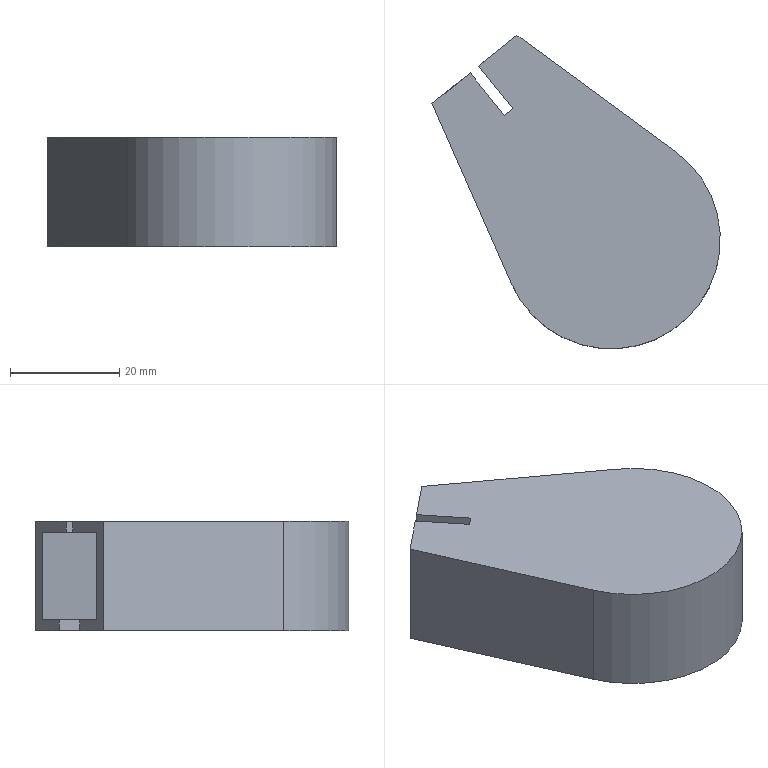Part | SolidWorks | features Cut 2, Extrusion 1, Shell 1 | 1 solid | 18 faces | box 52.852 x 57.443 x 20 mm | volume 11809 mm3 | plane 16 | cylinder 2 | commonest cylinder face diameters 36 x1 40 x1
STEP:
#1=CARTESIAN_POINT('',(-25.837,30.553,18.));
#2=VERTEX_POINT('',#1);
#3=CARTESIAN_POINT('',(-25.837,30.553,20.));
#4=VERTEX_POINT('',#3);
#5=CARTESIAN_POINT('',(-25.837,30.553,20.));
#6=DIRECTION('',(0.,0.,1.));
#7=VECTOR('',#6,1000.);
#8=LINE('',#5,#7);
#9=EDGE_CURVE('',#2,#4,#8,.T.);
#10=ORIENTED_EDGE('',*,*,#9,.F.);
#11=CARTESIAN_POINT('',(-31.238,26.212,18.));
#12=VERTEX_POINT('',#11);
#13=CARTESIAN_POINT('',(-25.057,31.179,18.));
#14=DIRECTION('',(0.7795,0.6264,0.));
#15=VECTOR('',#14,1000.);
#16=LINE('',#13,#15);
#17=EDGE_CURVE('',#12,#2,#16,.T.);
#18=ORIENTED_EDGE('',*,*,#17,.F.);
#19=CARTESIAN_POINT('',(-31.238,26.212,2.));
#20=VERTEX_POINT('',#19);
#21=CARTESIAN_POINT('',(-31.238,26.212,20.));
#22=DIRECTION('',(0.,0.,-1.));
#23=VECTOR('',#22,1000.);
#24=LINE('',#21,#23);
#25=EDGE_CURVE('',#12,#20,#24,.T.);
#26=ORIENTED_EDGE('',*,*,#25,.T.);
#27=CARTESIAN_POINT('',(-27.396,29.3,2.));
#28=VERTEX_POINT('',#27);
#29=CARTESIAN_POINT('',(-25.057,31.179,2.));
#30=DIRECTION('',(0.7795,0.6264,0.));
#31=VECTOR('',#30,1000.);
#32=LINE('',#29,#31);
#33=EDGE_CURVE('',#20,#28,#32,.T.);
#34=ORIENTED_EDGE('',*,*,#33,.T.);
#35=CARTESIAN_POINT('',(-27.396,29.3,0.));
#36=VERTEX_POINT('',#35);
#37=CARTESIAN_POINT('',(-27.396,29.3,20.001));
#38=DIRECTION('',(0.,0.,-1.));
#39=VECTOR('',#38,1000.);
#40=LINE('',#37,#39);
#41=EDGE_CURVE('',#28,#36,#40,.T.);
#42=ORIENTED_EDGE('',*,*,#41,.T.);
#43=CARTESIAN_POINT('',(-32.852,24.915,0.));
#44=VERTEX_POINT('',#43);
#45=CARTESIAN_POINT('',(-25.057,31.179,0.));
#46=DIRECTION('',(0.7795,0.6264,0.));
#47=VECTOR('',#46,1000.);
#48=LINE('',#45,#47);
#49=EDGE_CURVE('',#44,#36,#48,.T.);
#50=ORIENTED_EDGE('',*,*,#49,.F.);
#51=CARTESIAN_POINT('',(-32.852,24.915,20.));
#52=VERTEX_POINT('',#51);
#53=CARTESIAN_POINT('',(-32.852,24.915,20.));
#54=DIRECTION('',(0.,0.,-1.));
#55=VECTOR('',#54,1000.);
#56=LINE('',#53,#55);
#57=EDGE_CURVE('',#52,#44,#56,.T.);
#58=ORIENTED_EDGE('',*,*,#57,.F.);
#59=CARTESIAN_POINT('',(-25.057,31.179,20.));
#60=DIRECTION('',(0.7795,0.6264,0.));
#61=VECTOR('',#60,1000.);
#62=LINE('',#59,#61);
#63=EDGE_CURVE('',#52,#4,#62,.T.);
#64=ORIENTED_EDGE('',*,*,#63,.T.);
#65=EDGE_LOOP('',(#10,#18,#26,#34,#42,#50,#58,#64));
#66=FACE_OUTER_BOUND('',#65,.T.);
#67=CARTESIAN_POINT('',(-25.057,31.179,20.));
#68=DIRECTION('',(-0.6264,0.7795,0.));
#69=DIRECTION('',(-0.7795,-0.6264,0.));
#70=AXIS2_PLACEMENT_3D('',#67,#68,#69);
#71=PLANE('',#70);
#72=ADVANCED_FACE('',(#66),#71,.T.);
#73=CARTESIAN_POINT('',(-24.278,31.806,20.));
#74=VERTEX_POINT('',#73);
#75=CARTESIAN_POINT('',(-24.278,31.806,18.));
#76=VERTEX_POINT('',#75);
#77=CARTESIAN_POINT('',(-24.278,31.806,20.));
#78=DIRECTION('',(0.,0.,-1.));
#79=VECTOR('',#78,1000.);
#80=LINE('',#77,#79);
#81=EDGE_CURVE('',#74,#76,#80,.T.);
#82=ORIENTED_EDGE('',*,*,#81,.F.);
#83=CARTESIAN_POINT('',(-17.262,37.443,20.));
#84=VERTEX_POINT('',#83);
#85=CARTESIAN_POINT('',(-25.057,31.179,20.));
#86=DIRECTION('',(0.7795,0.6264,0.));
#87=VECTOR('',#86,1000.);
#88=LINE('',#85,#87);
#89=EDGE_CURVE('',#74,#84,#88,.T.);
#90=ORIENTED_EDGE('',*,*,#89,.T.);
#91=CARTESIAN_POINT('',(-17.262,37.443,0.));
#92=VERTEX_POINT('',#91);
#93=CARTESIAN_POINT('',(-17.262,37.443,20.));
#94=DIRECTION('',(0.,0.,-1.));
#95=VECTOR('',#94,1000.);
#96=LINE('',#93,#95);
#97=EDGE_CURVE('',#84,#92,#96,.T.);
#98=ORIENTED_EDGE('',*,*,#97,.T.);
#99=CARTESIAN_POINT('',(-22.719,33.058,0.));
#100=VERTEX_POINT('',#99);
#101=CARTESIAN_POINT('',(-25.057,31.179,0.));
#102=DIRECTION('',(0.7795,0.6264,0.));
#103=VECTOR('',#102,1000.);
#104=LINE('',#101,#103);
#105=EDGE_CURVE('',#100,#92,#104,.T.);
#106=ORIENTED_EDGE('',*,*,#105,.F.);
#107=CARTESIAN_POINT('',(-22.719,33.058,2.));
#108=VERTEX_POINT('',#107);
#109=CARTESIAN_POINT('',(-22.719,33.058,20.001));
#110=DIRECTION('',(0.,0.,1.));
#111=VECTOR('',#110,1000.);
#112=LINE('',#109,#111);
#113=EDGE_CURVE('',#100,#108,#112,.T.);
#114=ORIENTED_EDGE('',*,*,#113,.T.);
#115=CARTESIAN_POINT('',(-18.876,36.146,2.));
#116=VERTEX_POINT('',#115);
#117=CARTESIAN_POINT('',(-25.057,31.179,2.));
#118=DIRECTION('',(0.7795,0.6264,0.));
#119=VECTOR('',#118,1000.);
#120=LINE('',#117,#119);
#121=EDGE_CURVE('',#108,#116,#120,.T.);
#122=ORIENTED_EDGE('',*,*,#121,.T.);
#123=CARTESIAN_POINT('',(-18.876,36.146,18.));
#124=VERTEX_POINT('',#123);
#125=CARTESIAN_POINT('',(-18.876,36.146,20.));
#126=DIRECTION('',(0.,0.,-1.));
#127=VECTOR('',#126,1000.);
#128=LINE('',#125,#127);
#129=EDGE_CURVE('',#124,#116,#128,.T.);
#130=ORIENTED_EDGE('',*,*,#129,.F.);
#131=CARTESIAN_POINT('',(-25.057,31.179,18.));
#132=DIRECTION('',(0.7795,0.6264,0.));
#133=VECTOR('',#132,1000.);
#134=LINE('',#131,#133);
#135=EDGE_CURVE('',#76,#124,#134,.T.);
#136=ORIENTED_EDGE('',*,*,#135,.F.);
#137=EDGE_LOOP('',(#82,#90,#98,#106,#114,#122,#130,#136));
#138=FACE_OUTER_BOUND('',#137,.T.);
#139=CARTESIAN_POINT('',(-25.057,31.179,20.));
#140=DIRECTION('',(-0.6264,0.7795,0.));
#141=DIRECTION('',(-0.7795,-0.6264,0.));
#142=AXIS2_PLACEMENT_3D('',#139,#140,#141);
#143=PLANE('',#142);
#144=ADVANCED_FACE('',(#138),#143,.T.);
#145=CARTESIAN_POINT('',(-18.298,-8.073,0.));
#146=VERTEX_POINT('',#145);
#147=CARTESIAN_POINT('',(-18.298,-8.073,0.));
#148=DIRECTION('',(-0.4036,0.9149,0.));
#149=VECTOR('',#148,1000.);
#150=LINE('',#147,#149);
#151=EDGE_CURVE('',#146,#44,#150,.T.);
#152=ORIENTED_EDGE('',*,*,#151,.F.);
#153=CARTESIAN_POINT('',(-18.298,-8.073,20.));
#154=VERTEX_POINT('',#153);
#155=CARTESIAN_POINT('',(-18.298,-8.073,20.));
#156=DIRECTION('',(0.,0.,-1.));
#157=VECTOR('',#156,1000.);
#158=LINE('',#155,#157);
#159=EDGE_CURVE('',#154,#146,#158,.T.);
#160=ORIENTED_EDGE('',*,*,#159,.F.);
#161=CARTESIAN_POINT('',(-18.298,-8.073,20.));
#162=DIRECTION('',(-0.4036,0.9149,0.));
#163=VECTOR('',#162,1000.);
#164=LINE('',#161,#163);
#165=EDGE_CURVE('',#154,#52,#164,.T.);
#166=ORIENTED_EDGE('',*,*,#165,.T.);
#167=ORIENTED_EDGE('',*,*,#57,.T.);
#168=EDGE_LOOP('',(#152,#160,#166,#167));
#169=FACE_OUTER_BOUND('',#168,.T.);
#170=CARTESIAN_POINT('',(-18.298,-8.073,20.));
#171=DIRECTION('',(-0.9149,-0.4036,0.));
#172=DIRECTION('',(0.4036,-0.9149,0.));
#173=AXIS2_PLACEMENT_3D('',#170,#171,#172);
#174=PLANE('',#173);
#175=ADVANCED_FACE('',(#169),#174,.T.);
#176=CARTESIAN_POINT('',(11.821,16.133,0.));
#177=VERTEX_POINT('',#176);
#178=CARTESIAN_POINT('',(0.,0.,0.));
#179=DIRECTION('',(0.,0.,1.));
#180=DIRECTION('',(1.,0.,0.));
#181=AXIS2_PLACEMENT_3D('',#178,#179,#180);
#182=CIRCLE('',#181,20.);
#183=EDGE_CURVE('',#146,#177,#182,.T.);
#184=ORIENTED_EDGE('',*,*,#183,.T.);
#185=CARTESIAN_POINT('',(11.821,16.133,20.));
#186=VERTEX_POINT('',#185);
#187=CARTESIAN_POINT('',(11.821,16.133,20.));
#188=DIRECTION('',(0.,0.,-1.));
#189=VECTOR('',#188,1000.);
#190=LINE('',#187,#189);
#191=EDGE_CURVE('',#186,#177,#190,.T.);
#192=ORIENTED_EDGE('',*,*,#191,.F.);
#193=CARTESIAN_POINT('',(0.,0.,20.));
#194=DIRECTION('',(0.,0.,1.));
#195=DIRECTION('',(1.,0.,0.));
#196=AXIS2_PLACEMENT_3D('',#193,#194,#195);
#197=CIRCLE('',#196,20.);
#198=EDGE_CURVE('',#154,#186,#197,.T.);
#199=ORIENTED_EDGE('',*,*,#198,.F.);
#200=ORIENTED_EDGE('',*,*,#159,.T.);
#201=EDGE_LOOP('',(#184,#192,#199,#200));
#202=FACE_OUTER_BOUND('',#201,.T.);
#203=CARTESIAN_POINT('',(0.,0.,20.));
#204=DIRECTION('',(0.,0.,-1.));
#205=DIRECTION('',(-1.,0.,0.));
#206=AXIS2_PLACEMENT_3D('',#203,#204,#205);
#207=CYLINDRICAL_SURFACE('',#206,20.);
#208=ADVANCED_FACE('',(#202),#207,.T.);
#209=CARTESIAN_POINT('',(11.821,16.133,0.));
#210=DIRECTION('',(0.8066,-0.5911,0.));
#211=VECTOR('',#210,1000.);
#212=LINE('',#209,#211);
#213=EDGE_CURVE('',#92,#177,#212,.T.);
#214=ORIENTED_EDGE('',*,*,#213,.F.);
#215=ORIENTED_EDGE('',*,*,#97,.F.);
#216=CARTESIAN_POINT('',(11.821,16.133,20.));
#217=DIRECTION('',(0.8066,-0.5911,0.));
#218=VECTOR('',#217,1000.);
#219=LINE('',#216,#218);
#220=EDGE_CURVE('',#84,#186,#219,.T.);
#221=ORIENTED_EDGE('',*,*,#220,.T.);
#222=ORIENTED_EDGE('',*,*,#191,.T.);
#223=EDGE_LOOP('',(#214,#215,#221,#222));
#224=FACE_OUTER_BOUND('',#223,.T.);
#225=CARTESIAN_POINT('',(11.821,16.133,20.));
#226=DIRECTION('',(0.5911,0.8066,0.));
#227=DIRECTION('',(-0.8066,0.5911,0.));
#228=AXIS2_PLACEMENT_3D('',#225,#226,#227);
#229=PLANE('',#228);
#230=ADVANCED_FACE('',(#224),#229,.T.);
#231=CARTESIAN_POINT('',(-19.571,22.756,20.));
#232=VERTEX_POINT('',#231);
#233=CARTESIAN_POINT('',(-514.126,638.139,20.));
#234=DIRECTION('',(0.6264,-0.7795,0.));
#235=VECTOR('',#234,1000.);
#236=LINE('',#233,#235);
#237=EDGE_CURVE('',#4,#232,#236,.T.);
#238=ORIENTED_EDGE('',*,*,#237,.F.);
#239=ORIENTED_EDGE('',*,*,#63,.F.);
#240=ORIENTED_EDGE('',*,*,#165,.F.);
#241=ORIENTED_EDGE('',*,*,#198,.T.);
#242=ORIENTED_EDGE('',*,*,#220,.F.);
#243=ORIENTED_EDGE('',*,*,#89,.F.);
#244=CARTESIAN_POINT('',(-18.012,24.009,20.));
#245=VERTEX_POINT('',#244);
#246=CARTESIAN_POINT('',(-18.012,24.009,20.));
#247=DIRECTION('',(-0.6264,0.7795,0.));
#248=VECTOR('',#247,1000.);
#249=LINE('',#246,#248);
#250=EDGE_CURVE('',#245,#74,#249,.T.);
#251=ORIENTED_EDGE('',*,*,#250,.F.);
#252=CARTESIAN_POINT('',(-19.571,22.756,20.));
#253=DIRECTION('',(0.7795,0.6264,0.));
#254=VECTOR('',#253,1000.);
#255=LINE('',#252,#254);
#256=EDGE_CURVE('',#232,#245,#255,.T.);
#257=ORIENTED_EDGE('',*,*,#256,.F.);
#258=EDGE_LOOP('',(#238,#239,#240,#241,#242,#243,#251,#257));
#259=FACE_OUTER_BOUND('',#258,.T.);
#260=CARTESIAN_POINT('',(0.,0.,20.));
#261=DIRECTION('',(0.,0.,1.));
#262=DIRECTION('',(1.,0.,0.));
#263=AXIS2_PLACEMENT_3D('',#260,#261,#262);
#264=PLANE('',#263);
#265=ADVANCED_FACE('',(#259),#264,.T.);
#266=CARTESIAN_POINT('',(-16.454,25.264,0.));
#267=VERTEX_POINT('',#266);
#268=CARTESIAN_POINT('',(-21.131,21.505,0.));
#269=VERTEX_POINT('',#268);
#270=CARTESIAN_POINT('',(-21.131,21.505,0.));
#271=DIRECTION('',(-0.7795,-0.6264,0.));
#272=VECTOR('',#271,1000.);
#273=LINE('',#270,#272);
#274=EDGE_CURVE('',#267,#269,#273,.T.);
#275=ORIENTED_EDGE('',*,*,#274,.F.);
#276=CARTESIAN_POINT('',(-16.454,25.264,0.));
#277=DIRECTION('',(0.6264,-0.7795,0.));
#278=VECTOR('',#277,1000.);
#279=LINE('',#276,#278);
#280=EDGE_CURVE('',#100,#267,#279,.T.);
#281=ORIENTED_EDGE('',*,*,#280,.F.);
#282=ORIENTED_EDGE('',*,*,#105,.T.);
#283=ORIENTED_EDGE('',*,*,#213,.T.);
#284=ORIENTED_EDGE('',*,*,#183,.F.);
#285=ORIENTED_EDGE('',*,*,#151,.T.);
#286=ORIENTED_EDGE('',*,*,#49,.T.);
#287=CARTESIAN_POINT('',(-21.131,21.505,0.));
#288=DIRECTION('',(-0.6264,0.7795,0.));
#289=VECTOR('',#288,1000.);
#290=LINE('',#287,#289);
#291=EDGE_CURVE('',#269,#36,#290,.T.);
#292=ORIENTED_EDGE('',*,*,#291,.F.);
#293=EDGE_LOOP('',(#275,#281,#282,#283,#284,#285,#286,#292));
#294=FACE_OUTER_BOUND('',#293,.T.);
#295=CARTESIAN_POINT('',(0.,0.,0.));
#296=DIRECTION('',(0.,0.,1.));
#297=DIRECTION('',(1.,0.,0.));
#298=AXIS2_PLACEMENT_3D('',#295,#296,#297);
#299=PLANE('',#298);
#300=ADVANCED_FACE('',(#294),#299,.F.);
#301=CARTESIAN_POINT('',(-16.468,-7.266,2.));
#302=VERTEX_POINT('',#301);
#303=CARTESIAN_POINT('',(-16.468,-7.266,2.));
#304=DIRECTION('',(-0.4036,0.9149,0.));
#305=VECTOR('',#304,1000.);
#306=LINE('',#303,#305);
#307=EDGE_CURVE('',#302,#20,#306,.T.);
#308=ORIENTED_EDGE('',*,*,#307,.T.);
#309=ORIENTED_EDGE('',*,*,#25,.F.);
#310=CARTESIAN_POINT('',(-16.468,-7.266,18.));
#311=VERTEX_POINT('',#310);
#312=CARTESIAN_POINT('',(-16.468,-7.266,18.));
#313=DIRECTION('',(-0.4036,0.9149,0.));
#314=VECTOR('',#313,1000.);
#315=LINE('',#312,#314);
#316=EDGE_CURVE('',#311,#12,#315,.T.);
#317=ORIENTED_EDGE('',*,*,#316,.F.);
#318=CARTESIAN_POINT('',(-16.468,-7.266,20.));
#319=DIRECTION('',(0.,0.,-1.));
#320=VECTOR('',#319,1000.);
#321=LINE('',#318,#320);
#322=EDGE_CURVE('',#311,#302,#321,.T.);
#323=ORIENTED_EDGE('',*,*,#322,.T.);
#324=EDGE_LOOP('',(#308,#309,#317,#323));
#325=FACE_OUTER_BOUND('',#324,.T.);
#326=CARTESIAN_POINT('',(-16.468,-7.266,20.));
#327=DIRECTION('',(-0.9149,-0.4036,0.));
#328=DIRECTION('',(0.4036,-0.9149,0.));
#329=AXIS2_PLACEMENT_3D('',#326,#327,#328);
#330=PLANE('',#329);
#331=ADVANCED_FACE('',(#325),#330,.F.);
#332=CARTESIAN_POINT('',(10.639,14.519,2.));
#333=VERTEX_POINT('',#332);
#334=CARTESIAN_POINT('',(0.,0.,2.));
#335=DIRECTION('',(0.,0.,1.));
#336=DIRECTION('',(1.,0.,0.));
#337=AXIS2_PLACEMENT_3D('',#334,#335,#336);
#338=CIRCLE('',#337,18.);
#339=EDGE_CURVE('',#302,#333,#338,.T.);
#340=ORIENTED_EDGE('',*,*,#339,.F.);
#341=ORIENTED_EDGE('',*,*,#322,.F.);
#342=CARTESIAN_POINT('',(10.639,14.519,18.));
#343=VERTEX_POINT('',#342);
#344=CARTESIAN_POINT('',(0.,0.,18.));
#345=DIRECTION('',(0.,0.,1.));
#346=DIRECTION('',(1.,0.,0.));
#347=AXIS2_PLACEMENT_3D('',#344,#345,#346);
#348=CIRCLE('',#347,18.);
#349=EDGE_CURVE('',#311,#343,#348,.T.);
#350=ORIENTED_EDGE('',*,*,#349,.T.);
#351=CARTESIAN_POINT('',(10.639,14.519,20.));
#352=DIRECTION('',(0.,0.,-1.));
#353=VECTOR('',#352,1000.);
#354=LINE('',#351,#353);
#355=EDGE_CURVE('',#343,#333,#354,.T.);
#356=ORIENTED_EDGE('',*,*,#355,.T.);
#357=EDGE_LOOP('',(#340,#341,#350,#356));
#358=FACE_OUTER_BOUND('',#357,.T.);
#359=CARTESIAN_POINT('',(0.,0.,20.));
#360=DIRECTION('',(0.,0.,-1.));
#361=DIRECTION('',(-1.,0.,0.));
#362=AXIS2_PLACEMENT_3D('',#359,#360,#361);
#363=CYLINDRICAL_SURFACE('',#362,18.);
#364=ADVANCED_FACE('',(#358),#363,.F.);
#365=CARTESIAN_POINT('',(10.639,14.519,2.));
#366=DIRECTION('',(0.8066,-0.5911,0.));
#367=VECTOR('',#366,1000.);
#368=LINE('',#365,#367);
#369=EDGE_CURVE('',#116,#333,#368,.T.);
#370=ORIENTED_EDGE('',*,*,#369,.T.);
#371=ORIENTED_EDGE('',*,*,#355,.F.);
#372=CARTESIAN_POINT('',(10.639,14.519,18.));
#373=DIRECTION('',(0.8066,-0.5911,0.));
#374=VECTOR('',#373,1000.);
#375=LINE('',#372,#374);
#376=EDGE_CURVE('',#124,#343,#375,.T.);
#377=ORIENTED_EDGE('',*,*,#376,.F.);
#378=ORIENTED_EDGE('',*,*,#129,.T.);
#379=EDGE_LOOP('',(#370,#371,#377,#378));
#380=FACE_OUTER_BOUND('',#379,.T.);
#381=CARTESIAN_POINT('',(10.639,14.519,20.));
#382=DIRECTION('',(0.5911,0.8066,0.));
#383=DIRECTION('',(-0.8066,0.5911,0.));
#384=AXIS2_PLACEMENT_3D('',#381,#382,#383);
#385=PLANE('',#384);
#386=ADVANCED_FACE('',(#380),#385,.F.);
#387=ORIENTED_EDGE('',*,*,#17,.T.);
#388=CARTESIAN_POINT('',(-19.571,22.756,18.));
#389=VERTEX_POINT('',#388);
#390=CARTESIAN_POINT('',(-0.7795,-0.6264,18.));
#391=DIRECTION('',(0.6264,-0.7795,0.));
#392=VECTOR('',#391,1000.);
#393=LINE('',#390,#392);
#394=EDGE_CURVE('',#2,#389,#393,.T.);
#395=ORIENTED_EDGE('',*,*,#394,.T.);
#396=CARTESIAN_POINT('',(-18.012,24.009,18.));
#397=VERTEX_POINT('',#396);
#398=CARTESIAN_POINT('',(-18.791,23.382,18.));
#399=DIRECTION('',(0.7795,0.6264,0.));
#400=VECTOR('',#399,1000.);
#401=LINE('',#398,#400);
#402=EDGE_CURVE('',#389,#397,#401,.T.);
#403=ORIENTED_EDGE('',*,*,#402,.T.);
#404=CARTESIAN_POINT('',(0.7795,0.6264,18.));
#405=DIRECTION('',(-0.6264,0.7795,0.));
#406=VECTOR('',#405,1000.);
#407=LINE('',#404,#406);
#408=EDGE_CURVE('',#397,#76,#407,.T.);
#409=ORIENTED_EDGE('',*,*,#408,.T.);
#410=ORIENTED_EDGE('',*,*,#135,.T.);
#411=ORIENTED_EDGE('',*,*,#376,.T.);
#412=ORIENTED_EDGE('',*,*,#349,.F.);
#413=ORIENTED_EDGE('',*,*,#316,.T.);
#414=EDGE_LOOP('',(#387,#395,#403,#409,#410,#411,#412,#413));
#415=FACE_OUTER_BOUND('',#414,.T.);
#416=CARTESIAN_POINT('',(0.,0.,18.));
#417=DIRECTION('',(0.,0.,1.));
#418=DIRECTION('',(1.,0.,0.));
#419=AXIS2_PLACEMENT_3D('',#416,#417,#418);
#420=PLANE('',#419);
#421=ADVANCED_FACE('',(#415),#420,.F.);
#422=CARTESIAN_POINT('',(-16.454,25.264,2.));
#423=VERTEX_POINT('',#422);
#424=CARTESIAN_POINT('',(-21.131,21.505,2.));
#425=VERTEX_POINT('',#424);
#426=CARTESIAN_POINT('',(-21.131,21.505,2.));
#427=DIRECTION('',(-0.7795,-0.6264,0.));
#428=VECTOR('',#427,1000.);
#429=LINE('',#426,#428);
#430=EDGE_CURVE('',#423,#425,#429,.T.);
#431=ORIENTED_EDGE('',*,*,#430,.T.);
#432=CARTESIAN_POINT('',(-21.131,21.505,2.));
#433=DIRECTION('',(-0.6264,0.7795,0.));
#434=VECTOR('',#433,1000.);
#435=LINE('',#432,#434);
#436=EDGE_CURVE('',#425,#28,#435,.T.);
#437=ORIENTED_EDGE('',*,*,#436,.T.);
#438=ORIENTED_EDGE('',*,*,#33,.F.);
#439=ORIENTED_EDGE('',*,*,#307,.F.);
#440=ORIENTED_EDGE('',*,*,#339,.T.);
#441=ORIENTED_EDGE('',*,*,#369,.F.);
#442=ORIENTED_EDGE('',*,*,#121,.F.);
#443=CARTESIAN_POINT('',(-16.454,25.264,2.));
#444=DIRECTION('',(0.6264,-0.7795,0.));
#445=VECTOR('',#444,1000.);
#446=LINE('',#443,#445);
#447=EDGE_CURVE('',#108,#423,#446,.T.);
#448=ORIENTED_EDGE('',*,*,#447,.T.);
#449=EDGE_LOOP('',(#431,#437,#438,#439,#440,#441,#442,#448));
#450=FACE_OUTER_BOUND('',#449,.T.);
#451=CARTESIAN_POINT('',(0.,0.,2.));
#452=DIRECTION('',(0.,0.,1.));
#453=DIRECTION('',(1.,0.,0.));
#454=AXIS2_PLACEMENT_3D('',#451,#452,#453);
#455=PLANE('',#454);
#456=ADVANCED_FACE('',(#450),#455,.T.);
#457=ORIENTED_EDGE('',*,*,#280,.T.);
#458=CARTESIAN_POINT('',(-16.454,25.264,20.001));
#459=DIRECTION('',(0.,0.,-1.));
#460=VECTOR('',#459,1000.);
#461=LINE('',#458,#460);
#462=EDGE_CURVE('',#423,#267,#461,.T.);
#463=ORIENTED_EDGE('',*,*,#462,.F.);
#464=ORIENTED_EDGE('',*,*,#447,.F.);
#465=ORIENTED_EDGE('',*,*,#113,.F.);
#466=EDGE_LOOP('',(#457,#463,#464,#465));
#467=FACE_OUTER_BOUND('',#466,.T.);
#468=CARTESIAN_POINT('',(-16.454,25.264,20.001));
#469=DIRECTION('',(0.7795,0.6264,0.));
#470=DIRECTION('',(-0.6264,0.7795,0.));
#471=AXIS2_PLACEMENT_3D('',#468,#469,#470);
#472=PLANE('',#471);
#473=ADVANCED_FACE('',(#467),#472,.F.);
#474=ORIENTED_EDGE('',*,*,#462,.T.);
#475=ORIENTED_EDGE('',*,*,#274,.T.);
#476=CARTESIAN_POINT('',(-21.131,21.505,20.001));
#477=DIRECTION('',(0.,0.,-1.));
#478=VECTOR('',#477,1000.);
#479=LINE('',#476,#478);
#480=EDGE_CURVE('',#425,#269,#479,.T.);
#481=ORIENTED_EDGE('',*,*,#480,.F.);
#482=ORIENTED_EDGE('',*,*,#430,.F.);
#483=EDGE_LOOP('',(#474,#475,#481,#482));
#484=FACE_OUTER_BOUND('',#483,.T.);
#485=CARTESIAN_POINT('',(-21.131,21.505,20.001));
#486=DIRECTION('',(0.6264,-0.7795,0.));
#487=DIRECTION('',(0.7795,0.6264,0.));
#488=AXIS2_PLACEMENT_3D('',#485,#486,#487);
#489=PLANE('',#488);
#490=ADVANCED_FACE('',(#484),#489,.F.);
#491=ORIENTED_EDGE('',*,*,#436,.F.);
#492=ORIENTED_EDGE('',*,*,#480,.T.);
#493=ORIENTED_EDGE('',*,*,#291,.T.);
#494=ORIENTED_EDGE('',*,*,#41,.F.);
#495=EDGE_LOOP('',(#491,#492,#493,#494));
#496=FACE_OUTER_BOUND('',#495,.T.);
#497=CARTESIAN_POINT('',(-21.131,21.505,20.001));
#498=DIRECTION('',(-0.7795,-0.6264,0.));
#499=DIRECTION('',(0.6264,-0.7795,0.));
#500=AXIS2_PLACEMENT_3D('',#497,#498,#499);
#501=PLANE('',#500);
#502=ADVANCED_FACE('',(#496),#501,.F.);
#503=CARTESIAN_POINT('',(-19.571,22.756,-789.435));
#504=DIRECTION('',(0.,0.,1.));
#505=VECTOR('',#504,1000.);
#506=LINE('',#503,#505);
#507=EDGE_CURVE('',#389,#232,#506,.T.);
#508=ORIENTED_EDGE('',*,*,#507,.T.);
#509=ORIENTED_EDGE('',*,*,#256,.T.);
#510=CARTESIAN_POINT('',(-18.012,24.009,-789.435));
#511=DIRECTION('',(0.,0.,1.));
#512=VECTOR('',#511,1000.);
#513=LINE('',#510,#512);
#514=EDGE_CURVE('',#397,#245,#513,.T.);
#515=ORIENTED_EDGE('',*,*,#514,.F.);
#516=ORIENTED_EDGE('',*,*,#402,.F.);
#517=EDGE_LOOP('',(#508,#509,#515,#516));
#518=FACE_OUTER_BOUND('',#517,.T.);
#519=CARTESIAN_POINT('',(-19.571,22.756,-789.435));
#520=DIRECTION('',(0.6264,-0.7795,0.));
#521=DIRECTION('',(0.7795,0.6264,0.));
#522=AXIS2_PLACEMENT_3D('',#519,#520,#521);
#523=PLANE('',#522);
#524=ADVANCED_FACE('',(#518),#523,.F.);
#525=ORIENTED_EDGE('',*,*,#9,.T.);
#526=ORIENTED_EDGE('',*,*,#237,.T.);
#527=ORIENTED_EDGE('',*,*,#507,.F.);
#528=ORIENTED_EDGE('',*,*,#394,.F.);
#529=EDGE_LOOP('',(#525,#526,#527,#528));
#530=FACE_OUTER_BOUND('',#529,.T.);
#531=CARTESIAN_POINT('',(-514.126,638.139,-789.435));
#532=DIRECTION('',(-0.7795,-0.6264,0.));
#533=DIRECTION('',(0.6264,-0.7795,0.));
#534=AXIS2_PLACEMENT_3D('',#531,#532,#533);
#535=PLANE('',#534);
#536=ADVANCED_FACE('',(#530),#535,.F.);
#537=ORIENTED_EDGE('',*,*,#81,.T.);
#538=ORIENTED_EDGE('',*,*,#408,.F.);
#539=ORIENTED_EDGE('',*,*,#514,.T.);
#540=ORIENTED_EDGE('',*,*,#250,.T.);
#541=EDGE_LOOP('',(#537,#538,#539,#540));
#542=FACE_OUTER_BOUND('',#541,.T.);
#543=CARTESIAN_POINT('',(-18.012,24.009,-789.435));
#544=DIRECTION('',(0.7795,0.6264,0.));
#545=DIRECTION('',(-0.6264,0.7795,0.));
#546=AXIS2_PLACEMENT_3D('',#543,#544,#545);
#547=PLANE('',#546);
#548=ADVANCED_FACE('',(#542),#547,.F.);
#549=CLOSED_SHELL('',(#72,#144,#175,#208,#230,#265,#300,#331,#364,#386,#421,#456,#473,#490,#502,#524,#536,#548));
#550=MANIFOLD_SOLID_BREP('',#549);
#551=CARTESIAN_POINT('',(0.,0.,0.));
#552=DIRECTION('',(0.,0.,1.));
#553=DIRECTION('',(1.,0.,0.));
#554=AXIS2_PLACEMENT_3D('',#551,#552,#553);
#555=(LENGTH_UNIT()NAMED_UNIT(*)SI_UNIT(.MILLI.,.METRE.));
#556=UNCERTAINTY_MEASURE_WITH_UNIT(LENGTH_MEASURE(0.00001),#555,'','');
#557=(NAMED_UNIT(*)PLANE_ANGLE_UNIT()SI_UNIT($,.RADIAN.));
#558=(NAMED_UNIT(*)SI_UNIT($,.STERADIAN.)SOLID_ANGLE_UNIT());
#559=(GEOMETRIC_REPRESENTATION_CONTEXT(3)GLOBAL_UNCERTAINTY_ASSIGNED_CONTEXT((#556))GLOBAL_UNIT_ASSIGNED_CONTEXT((#555,#557,#558))REPRESENTATION_CONTEXT('',''));
#560=ADVANCED_BREP_SHAPE_REPRESENTATION('',(#550,#554),#559);